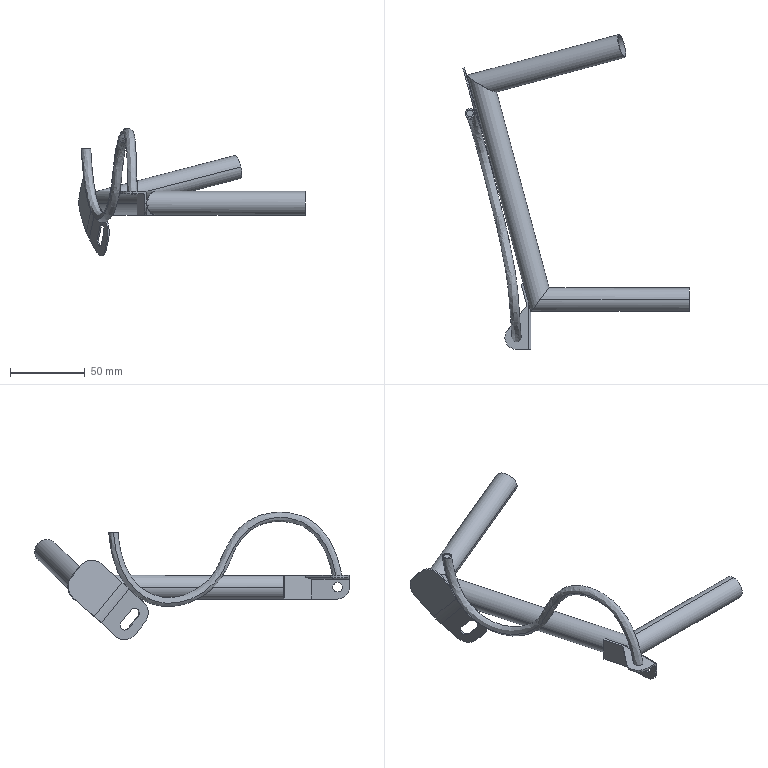Part | SolidWorks | features BaseBody 7 | 7 solids | 64 faces | box 151.634 x 211.019 x 85.41 mm | volume 28797 mm3 | cylinder 30 | plane 30 | spline 4 | commonest cylinder face diameters 15.875 x8 14.097 x6 20 x5 7 x3 3.048 x2 5.204 x2